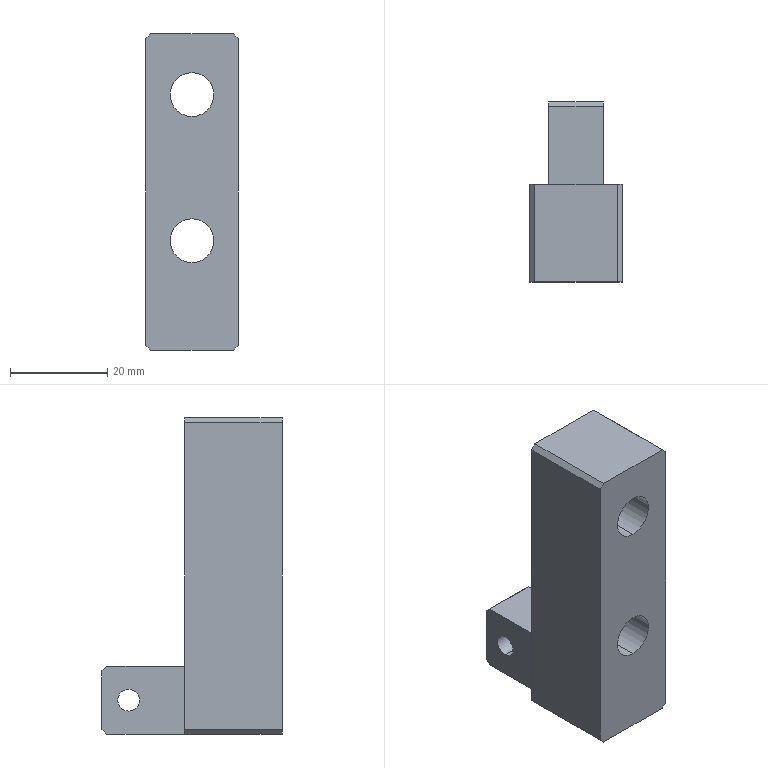Part | STEP file | Fixing block 1 | 1 solid | 28 faces | box 19 x 37 x 65 mm | volume 22556 mm3 | plane 18 | cylinder 10 | commonest cylinder face diameters 9 x4 15 x4 4.5 x2